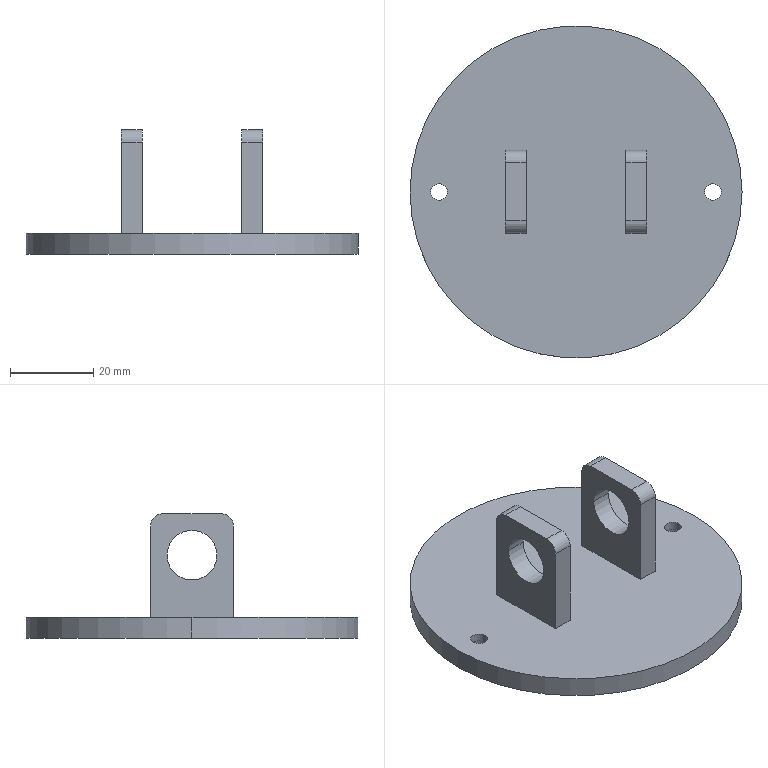Part | STEP file | Hinge seat 1 | 1 solid | 32 faces | box 80 x 80 x 30 mm | volume 28682 mm3 | cylinder 18 | plane 14 | commonest cylinder face diameters 4 x4 6 x4 7 x4 12 x4 80 x2
STEP:
#1=CARTESIAN_POINT('',(-29.5,0.,3.));
#2=VERTEX_POINT('',#1);
#3=CARTESIAN_POINT('',(-36.5,0.,3.));
#4=VERTEX_POINT('',#3);
#5=CARTESIAN_POINT('',(-33.,0.,3.));
#6=DIRECTION('',(0.,0.,-1.));
#7=DIRECTION('',(-1.,0.,0.));
#8=AXIS2_PLACEMENT_3D('',#5,#6,#7);
#9=CIRCLE('',#8,3.5);
#10=EDGE_CURVE('',#2,#4,#9,.T.);
#11=ORIENTED_EDGE('',*,*,#10,.F.);
#12=CARTESIAN_POINT('',(-29.5,0.,0.));
#13=VERTEX_POINT('',#12);
#14=CARTESIAN_POINT('',(-29.5,0.,3.));
#15=DIRECTION('',(0.,0.,-1.));
#16=VECTOR('',#15,1000.);
#17=LINE('',#14,#16);
#18=EDGE_CURVE('',#2,#13,#17,.T.);
#19=ORIENTED_EDGE('',*,*,#18,.T.);
#20=CARTESIAN_POINT('',(-36.5,0.,0.));
#21=VERTEX_POINT('',#20);
#22=CARTESIAN_POINT('',(-33.,0.,0.));
#23=DIRECTION('',(0.,0.,-1.));
#24=DIRECTION('',(-1.,0.,0.));
#25=AXIS2_PLACEMENT_3D('',#22,#23,#24);
#26=CIRCLE('',#25,3.5);
#27=EDGE_CURVE('',#13,#21,#26,.T.);
#28=ORIENTED_EDGE('',*,*,#27,.T.);
#29=CARTESIAN_POINT('',(-36.5,0.,3.));
#30=DIRECTION('',(0.,0.,-1.));
#31=VECTOR('',#30,1000.);
#32=LINE('',#29,#31);
#33=EDGE_CURVE('',#4,#21,#32,.T.);
#34=ORIENTED_EDGE('',*,*,#33,.F.);
#35=EDGE_LOOP('',(#11,#19,#28,#34));
#36=FACE_OUTER_BOUND('',#35,.T.);
#37=CARTESIAN_POINT('',(-33.,0.,3.));
#38=DIRECTION('',(0.,0.,-1.));
#39=DIRECTION('',(-1.,0.,0.));
#40=AXIS2_PLACEMENT_3D('',#37,#38,#39);
#41=CYLINDRICAL_SURFACE('',#40,3.5);
#42=ADVANCED_FACE('',(#36),#41,.F.);
#43=CARTESIAN_POINT('',(36.5,0.,3.));
#44=VERTEX_POINT('',#43);
#45=CARTESIAN_POINT('',(29.5,0.,3.));
#46=VERTEX_POINT('',#45);
#47=CARTESIAN_POINT('',(33.,0.,3.));
#48=DIRECTION('',(0.,0.,-1.));
#49=DIRECTION('',(-1.,0.,0.));
#50=AXIS2_PLACEMENT_3D('',#47,#48,#49);
#51=CIRCLE('',#50,3.5);
#52=EDGE_CURVE('',#44,#46,#51,.T.);
#53=ORIENTED_EDGE('',*,*,#52,.F.);
#54=CARTESIAN_POINT('',(36.5,0.,0.));
#55=VERTEX_POINT('',#54);
#56=CARTESIAN_POINT('',(36.5,0.,3.));
#57=DIRECTION('',(0.,0.,-1.));
#58=VECTOR('',#57,1000.);
#59=LINE('',#56,#58);
#60=EDGE_CURVE('',#44,#55,#59,.T.);
#61=ORIENTED_EDGE('',*,*,#60,.T.);
#62=CARTESIAN_POINT('',(29.5,0.,0.));
#63=VERTEX_POINT('',#62);
#64=CARTESIAN_POINT('',(33.,0.,0.));
#65=DIRECTION('',(0.,0.,-1.));
#66=DIRECTION('',(-1.,0.,0.));
#67=AXIS2_PLACEMENT_3D('',#64,#65,#66);
#68=CIRCLE('',#67,3.5);
#69=EDGE_CURVE('',#55,#63,#68,.T.);
#70=ORIENTED_EDGE('',*,*,#69,.T.);
#71=CARTESIAN_POINT('',(29.5,0.,3.));
#72=DIRECTION('',(0.,0.,-1.));
#73=VECTOR('',#72,1000.);
#74=LINE('',#71,#73);
#75=EDGE_CURVE('',#46,#63,#74,.T.);
#76=ORIENTED_EDGE('',*,*,#75,.F.);
#77=EDGE_LOOP('',(#53,#61,#70,#76));
#78=FACE_OUTER_BOUND('',#77,.T.);
#79=CARTESIAN_POINT('',(33.,0.,3.));
#80=DIRECTION('',(0.,0.,-1.));
#81=DIRECTION('',(-1.,0.,0.));
#82=AXIS2_PLACEMENT_3D('',#79,#80,#81);
#83=CYLINDRICAL_SURFACE('',#82,3.5);
#84=ADVANCED_FACE('',(#78),#83,.F.);
#85=CARTESIAN_POINT('',(-12.,6.,20.));
#86=VERTEX_POINT('',#85);
#87=CARTESIAN_POINT('',(-12.,-6.,20.));
#88=VERTEX_POINT('',#87);
#89=CARTESIAN_POINT('',(-12.,0.,20.));
#90=DIRECTION('',(-1.,0.,0.));
#91=DIRECTION('',(0.,-1.,0.));
#92=AXIS2_PLACEMENT_3D('',#89,#90,#91);
#93=CIRCLE('',#92,6.);
#94=EDGE_CURVE('',#86,#88,#93,.T.);
#95=ORIENTED_EDGE('',*,*,#94,.F.);
#96=CARTESIAN_POINT('',(-17.,6.,20.));
#97=VERTEX_POINT('',#96);
#98=CARTESIAN_POINT('',(40.,6.,20.));
#99=DIRECTION('',(-1.,0.,0.));
#100=VECTOR('',#99,1000.);
#101=LINE('',#98,#100);
#102=EDGE_CURVE('',#86,#97,#101,.T.);
#103=ORIENTED_EDGE('',*,*,#102,.T.);
#104=CARTESIAN_POINT('',(-17.,-6.,20.));
#105=VERTEX_POINT('',#104);
#106=CARTESIAN_POINT('',(-17.,0.,20.));
#107=DIRECTION('',(-1.,0.,0.));
#108=DIRECTION('',(0.,-1.,0.));
#109=AXIS2_PLACEMENT_3D('',#106,#107,#108);
#110=CIRCLE('',#109,6.);
#111=EDGE_CURVE('',#97,#105,#110,.T.);
#112=ORIENTED_EDGE('',*,*,#111,.T.);
#113=CARTESIAN_POINT('',(40.,-6.,20.));
#114=DIRECTION('',(-1.,0.,0.));
#115=VECTOR('',#114,1000.);
#116=LINE('',#113,#115);
#117=EDGE_CURVE('',#88,#105,#116,.T.);
#118=ORIENTED_EDGE('',*,*,#117,.F.);
#119=EDGE_LOOP('',(#95,#103,#112,#118));
#120=FACE_OUTER_BOUND('',#119,.T.);
#121=CARTESIAN_POINT('',(40.,0.,20.));
#122=DIRECTION('',(-1.,0.,0.));
#123=DIRECTION('',(0.,-1.,0.));
#124=AXIS2_PLACEMENT_3D('',#121,#122,#123);
#125=CYLINDRICAL_SURFACE('',#124,6.);
#126=ADVANCED_FACE('',(#120),#125,.F.);
#127=CARTESIAN_POINT('',(17.,6.,20.));
#128=VERTEX_POINT('',#127);
#129=CARTESIAN_POINT('',(17.,-6.,20.));
#130=VERTEX_POINT('',#129);
#131=CARTESIAN_POINT('',(17.,0.,20.));
#132=DIRECTION('',(-1.,0.,0.));
#133=DIRECTION('',(0.,-1.,0.));
#134=AXIS2_PLACEMENT_3D('',#131,#132,#133);
#135=CIRCLE('',#134,6.);
#136=EDGE_CURVE('',#128,#130,#135,.T.);
#137=ORIENTED_EDGE('',*,*,#136,.F.);
#138=CARTESIAN_POINT('',(12.,6.,20.));
#139=VERTEX_POINT('',#138);
#140=CARTESIAN_POINT('',(40.,6.,20.));
#141=DIRECTION('',(-1.,0.,0.));
#142=VECTOR('',#141,1000.);
#143=LINE('',#140,#142);
#144=EDGE_CURVE('',#128,#139,#143,.T.);
#145=ORIENTED_EDGE('',*,*,#144,.T.);
#146=CARTESIAN_POINT('',(12.,-6.,20.));
#147=VERTEX_POINT('',#146);
#148=CARTESIAN_POINT('',(12.,0.,20.));
#149=DIRECTION('',(1.,0.,0.));
#150=DIRECTION('',(0.,1.,0.));
#151=AXIS2_PLACEMENT_3D('',#148,#149,#150);
#152=CIRCLE('',#151,6.);
#153=EDGE_CURVE('',#147,#139,#152,.T.);
#154=ORIENTED_EDGE('',*,*,#153,.F.);
#155=CARTESIAN_POINT('',(40.,-6.,20.));
#156=DIRECTION('',(-1.,0.,0.));
#157=VECTOR('',#156,1000.);
#158=LINE('',#155,#157);
#159=EDGE_CURVE('',#130,#147,#158,.T.);
#160=ORIENTED_EDGE('',*,*,#159,.F.);
#161=EDGE_LOOP('',(#137,#145,#154,#160));
#162=FACE_OUTER_BOUND('',#161,.T.);
#163=CARTESIAN_POINT('',(40.,0.,20.));
#164=DIRECTION('',(-1.,0.,0.));
#165=DIRECTION('',(0.,-1.,0.));
#166=AXIS2_PLACEMENT_3D('',#163,#164,#165);
#167=CYLINDRICAL_SURFACE('',#166,6.);
#168=ADVANCED_FACE('',(#162),#167,.F.);
#169=CARTESIAN_POINT('',(40.,0.,5.));
#170=VERTEX_POINT('',#169);
#171=CARTESIAN_POINT('',(-40.,0.,5.));
#172=VERTEX_POINT('',#171);
#173=CARTESIAN_POINT('',(0.,0.,5.));
#174=DIRECTION('',(0.,0.,1.));
#175=DIRECTION('',(1.,0.,0.));
#176=AXIS2_PLACEMENT_3D('',#173,#174,#175);
#177=CIRCLE('',#176,40.);
#178=EDGE_CURVE('',#170,#172,#177,.T.);
#179=ORIENTED_EDGE('',*,*,#178,.F.);
#180=CARTESIAN_POINT('',(40.,0.,0.));
#181=VERTEX_POINT('',#180);
#182=CARTESIAN_POINT('',(40.,0.,5.));
#183=DIRECTION('',(0.,0.,-1.));
#184=VECTOR('',#183,1000.);
#185=LINE('',#182,#184);
#186=EDGE_CURVE('',#170,#181,#185,.T.);
#187=ORIENTED_EDGE('',*,*,#186,.T.);
#188=CARTESIAN_POINT('',(-40.,0.,0.));
#189=VERTEX_POINT('',#188);
#190=CARTESIAN_POINT('',(0.,0.,0.));
#191=DIRECTION('',(0.,0.,1.));
#192=DIRECTION('',(1.,0.,0.));
#193=AXIS2_PLACEMENT_3D('',#190,#191,#192);
#194=CIRCLE('',#193,40.);
#195=EDGE_CURVE('',#181,#189,#194,.T.);
#196=ORIENTED_EDGE('',*,*,#195,.T.);
#197=CARTESIAN_POINT('',(-40.,0.,5.));
#198=DIRECTION('',(0.,0.,-1.));
#199=VECTOR('',#198,1000.);
#200=LINE('',#197,#199);
#201=EDGE_CURVE('',#172,#189,#200,.T.);
#202=ORIENTED_EDGE('',*,*,#201,.F.);
#203=EDGE_LOOP('',(#179,#187,#196,#202));
#204=FACE_OUTER_BOUND('',#203,.T.);
#205=CARTESIAN_POINT('',(0.,0.,5.));
#206=DIRECTION('',(0.,0.,-1.));
#207=DIRECTION('',(-1.,0.,0.));
#208=AXIS2_PLACEMENT_3D('',#205,#206,#207);
#209=CYLINDRICAL_SURFACE('',#208,40.);
#210=ADVANCED_FACE('',(#204),#209,.T.);
#211=CARTESIAN_POINT('',(31.,0.,5.));
#212=VERTEX_POINT('',#211);
#213=CARTESIAN_POINT('',(35.,0.,5.));
#214=VERTEX_POINT('',#213);
#215=CARTESIAN_POINT('',(33.,0.,5.));
#216=DIRECTION('',(0.,0.,1.));
#217=DIRECTION('',(1.,0.,0.));
#218=AXIS2_PLACEMENT_3D('',#215,#216,#217);
#219=CIRCLE('',#218,2.);
#220=EDGE_CURVE('',#212,#214,#219,.T.);
#221=ORIENTED_EDGE('',*,*,#220,.T.);
#222=CARTESIAN_POINT('',(35.,0.,3.));
#223=VERTEX_POINT('',#222);
#224=CARTESIAN_POINT('',(35.,0.,30.));
#225=DIRECTION('',(0.,0.,-1.));
#226=VECTOR('',#225,1000.);
#227=LINE('',#224,#226);
#228=EDGE_CURVE('',#214,#223,#227,.T.);
#229=ORIENTED_EDGE('',*,*,#228,.T.);
#230=CARTESIAN_POINT('',(31.,0.,3.));
#231=VERTEX_POINT('',#230);
#232=CARTESIAN_POINT('',(33.,0.,3.));
#233=DIRECTION('',(0.,0.,1.));
#234=DIRECTION('',(-1.,0.,0.));
#235=AXIS2_PLACEMENT_3D('',#232,#233,#234);
#236=CIRCLE('',#235,2.);
#237=EDGE_CURVE('',#231,#223,#236,.T.);
#238=ORIENTED_EDGE('',*,*,#237,.F.);
#239=CARTESIAN_POINT('',(31.,0.,30.));
#240=DIRECTION('',(0.,0.,-1.));
#241=VECTOR('',#240,1000.);
#242=LINE('',#239,#241);
#243=EDGE_CURVE('',#212,#231,#242,.T.);
#244=ORIENTED_EDGE('',*,*,#243,.F.);
#245=EDGE_LOOP('',(#221,#229,#238,#244));
#246=FACE_OUTER_BOUND('',#245,.T.);
#247=CARTESIAN_POINT('',(33.,0.,30.));
#248=DIRECTION('',(0.,0.,-1.));
#249=DIRECTION('',(-1.,0.,0.));
#250=AXIS2_PLACEMENT_3D('',#247,#248,#249);
#251=CYLINDRICAL_SURFACE('',#250,2.);
#252=ADVANCED_FACE('',(#246),#251,.F.);
#253=CARTESIAN_POINT('',(-35.,0.,5.));
#254=VERTEX_POINT('',#253);
#255=CARTESIAN_POINT('',(-31.,0.,5.));
#256=VERTEX_POINT('',#255);
#257=CARTESIAN_POINT('',(-33.,0.,5.));
#258=DIRECTION('',(0.,0.,1.));
#259=DIRECTION('',(1.,0.,0.));
#260=AXIS2_PLACEMENT_3D('',#257,#258,#259);
#261=CIRCLE('',#260,2.);
#262=EDGE_CURVE('',#254,#256,#261,.T.);
#263=ORIENTED_EDGE('',*,*,#262,.T.);
#264=CARTESIAN_POINT('',(-31.,0.,3.));
#265=VERTEX_POINT('',#264);
#266=CARTESIAN_POINT('',(-31.,0.,30.));
#267=DIRECTION('',(0.,0.,-1.));
#268=VECTOR('',#267,1000.);
#269=LINE('',#266,#268);
#270=EDGE_CURVE('',#256,#265,#269,.T.);
#271=ORIENTED_EDGE('',*,*,#270,.T.);
#272=CARTESIAN_POINT('',(-35.,0.,3.));
#273=VERTEX_POINT('',#272);
#274=CARTESIAN_POINT('',(-33.,0.,3.));
#275=DIRECTION('',(0.,0.,1.));
#276=DIRECTION('',(-1.,0.,0.));
#277=AXIS2_PLACEMENT_3D('',#274,#275,#276);
#278=CIRCLE('',#277,2.);
#279=EDGE_CURVE('',#273,#265,#278,.T.);
#280=ORIENTED_EDGE('',*,*,#279,.F.);
#281=CARTESIAN_POINT('',(-35.,0.,30.));
#282=DIRECTION('',(0.,0.,-1.));
#283=VECTOR('',#282,1000.);
#284=LINE('',#281,#283);
#285=EDGE_CURVE('',#254,#273,#284,.T.);
#286=ORIENTED_EDGE('',*,*,#285,.F.);
#287=EDGE_LOOP('',(#263,#271,#280,#286));
#288=FACE_OUTER_BOUND('',#287,.T.);
#289=CARTESIAN_POINT('',(-33.,0.,30.));
#290=DIRECTION('',(0.,0.,-1.));
#291=DIRECTION('',(-1.,0.,0.));
#292=AXIS2_PLACEMENT_3D('',#289,#290,#291);
#293=CYLINDRICAL_SURFACE('',#292,2.);
#294=ADVANCED_FACE('',(#288),#293,.F.);
#295=ORIENTED_EDGE('',*,*,#270,.F.);
#296=CARTESIAN_POINT('',(-33.,0.,5.));
#297=DIRECTION('',(0.,0.,1.));
#298=DIRECTION('',(1.,0.,0.));
#299=AXIS2_PLACEMENT_3D('',#296,#297,#298);
#300=CIRCLE('',#299,2.);
#301=EDGE_CURVE('',#256,#254,#300,.T.);
#302=ORIENTED_EDGE('',*,*,#301,.T.);
#303=ORIENTED_EDGE('',*,*,#285,.T.);
#304=CARTESIAN_POINT('',(-33.,0.,3.));
#305=DIRECTION('',(0.,0.,1.));
#306=DIRECTION('',(-1.,0.,0.));
#307=AXIS2_PLACEMENT_3D('',#304,#305,#306);
#308=CIRCLE('',#307,2.);
#309=EDGE_CURVE('',#265,#273,#308,.T.);
#310=ORIENTED_EDGE('',*,*,#309,.F.);
#311=EDGE_LOOP('',(#295,#302,#303,#310));
#312=FACE_OUTER_BOUND('',#311,.T.);
#313=CARTESIAN_POINT('',(-33.,0.,30.));
#314=DIRECTION('',(0.,0.,-1.));
#315=DIRECTION('',(-1.,0.,0.));
#316=AXIS2_PLACEMENT_3D('',#313,#314,#315);
#317=CYLINDRICAL_SURFACE('',#316,2.);
#318=ADVANCED_FACE('',(#312),#317,.F.);
#319=ORIENTED_EDGE('',*,*,#228,.F.);
#320=CARTESIAN_POINT('',(33.,0.,5.));
#321=DIRECTION('',(0.,0.,1.));
#322=DIRECTION('',(1.,0.,0.));
#323=AXIS2_PLACEMENT_3D('',#320,#321,#322);
#324=CIRCLE('',#323,2.);
#325=EDGE_CURVE('',#214,#212,#324,.T.);
#326=ORIENTED_EDGE('',*,*,#325,.T.);
#327=ORIENTED_EDGE('',*,*,#243,.T.);
#328=CARTESIAN_POINT('',(33.,0.,3.));
#329=DIRECTION('',(0.,0.,1.));
#330=DIRECTION('',(-1.,0.,0.));
#331=AXIS2_PLACEMENT_3D('',#328,#329,#330);
#332=CIRCLE('',#331,2.);
#333=EDGE_CURVE('',#223,#231,#332,.T.);
#334=ORIENTED_EDGE('',*,*,#333,.F.);
#335=EDGE_LOOP('',(#319,#326,#327,#334));
#336=FACE_OUTER_BOUND('',#335,.T.);
#337=CARTESIAN_POINT('',(33.,0.,30.));
#338=DIRECTION('',(0.,0.,-1.));
#339=DIRECTION('',(-1.,0.,0.));
#340=AXIS2_PLACEMENT_3D('',#337,#338,#339);
#341=CYLINDRICAL_SURFACE('',#340,2.);
#342=ADVANCED_FACE('',(#336),#341,.F.);
#343=ORIENTED_EDGE('',*,*,#220,.F.);
#344=ORIENTED_EDGE('',*,*,#325,.F.);
#345=EDGE_LOOP('',(#343,#344));
#346=FACE_BOUND('',#345,.T.);
#347=ORIENTED_EDGE('',*,*,#262,.F.);
#348=ORIENTED_EDGE('',*,*,#301,.F.);
#349=EDGE_LOOP('',(#347,#348));
#350=FACE_BOUND('',#349,.T.);
#351=CARTESIAN_POINT('',(0.,0.,5.));
#352=DIRECTION('',(0.,0.,1.));
#353=DIRECTION('',(1.,0.,0.));
#354=AXIS2_PLACEMENT_3D('',#351,#352,#353);
#355=CIRCLE('',#354,40.);
#356=EDGE_CURVE('',#172,#170,#355,.T.);
#357=ORIENTED_EDGE('',*,*,#356,.T.);
#358=ORIENTED_EDGE('',*,*,#178,.T.);
#359=EDGE_LOOP('',(#357,#358));
#360=FACE_OUTER_BOUND('',#359,.T.);
#361=CARTESIAN_POINT('',(-12.,10.,5.));
#362=VERTEX_POINT('',#361);
#363=CARTESIAN_POINT('',(-17.,10.,5.));
#364=VERTEX_POINT('',#363);
#365=CARTESIAN_POINT('',(-17.,10.,5.));
#366=DIRECTION('',(-1.,0.,0.));
#367=VECTOR('',#366,1000.);
#368=LINE('',#365,#367);
#369=EDGE_CURVE('',#362,#364,#368,.T.);
#370=ORIENTED_EDGE('',*,*,#369,.F.);
#371=CARTESIAN_POINT('',(-12.,-10.,5.));
#372=VERTEX_POINT('',#371);
#373=CARTESIAN_POINT('',(-12.,10.,5.));
#374=DIRECTION('',(0.,1.,0.));
#375=VECTOR('',#374,1000.);
#376=LINE('',#373,#375);
#377=EDGE_CURVE('',#372,#362,#376,.T.);
#378=ORIENTED_EDGE('',*,*,#377,.F.);
#379=CARTESIAN_POINT('',(-17.,-10.,5.));
#380=VERTEX_POINT('',#379);
#381=CARTESIAN_POINT('',(-17.,-10.,5.));
#382=DIRECTION('',(1.,0.,0.));
#383=VECTOR('',#382,1000.);
#384=LINE('',#381,#383);
#385=EDGE_CURVE('',#380,#372,#384,.T.);
#386=ORIENTED_EDGE('',*,*,#385,.F.);
#387=CARTESIAN_POINT('',(-17.,10.,5.));
#388=DIRECTION('',(0.,-1.,0.));
#389=VECTOR('',#388,1000.);
#390=LINE('',#387,#389);
#391=EDGE_CURVE('',#364,#380,#390,.T.);
#392=ORIENTED_EDGE('',*,*,#391,.F.);
#393=EDGE_LOOP('',(#370,#378,#386,#392));
#394=FACE_BOUND('',#393,.T.);
#395=CARTESIAN_POINT('',(17.,10.,5.));
#396=VERTEX_POINT('',#395);
#397=CARTESIAN_POINT('',(12.,10.,5.));
#398=VERTEX_POINT('',#397);
#399=CARTESIAN_POINT('',(17.,10.,5.));
#400=DIRECTION('',(-1.,0.,0.));
#401=VECTOR('',#400,1000.);
#402=LINE('',#399,#401);
#403=EDGE_CURVE('',#396,#398,#402,.T.);
#404=ORIENTED_EDGE('',*,*,#403,.F.);
#405=CARTESIAN_POINT('',(17.,-10.,5.));
#406=VERTEX_POINT('',#405);
#407=CARTESIAN_POINT('',(17.,10.,5.));
#408=DIRECTION('',(0.,1.,0.));
#409=VECTOR('',#408,1000.);
#410=LINE('',#407,#409);
#411=EDGE_CURVE('',#406,#396,#410,.T.);
#412=ORIENTED_EDGE('',*,*,#411,.F.);
#413=CARTESIAN_POINT('',(12.,-10.,5.));
#414=VERTEX_POINT('',#413);
#415=CARTESIAN_POINT('',(17.,-10.,5.));
#416=DIRECTION('',(1.,0.,0.));
#417=VECTOR('',#416,1000.);
#418=LINE('',#415,#417);
#419=EDGE_CURVE('',#414,#406,#418,.T.);
#420=ORIENTED_EDGE('',*,*,#419,.F.);
#421=CARTESIAN_POINT('',(12.,10.,5.));
#422=DIRECTION('',(0.,-1.,0.));
#423=VECTOR('',#422,1000.);
#424=LINE('',#421,#423);
#425=EDGE_CURVE('',#398,#414,#424,.T.);
#426=ORIENTED_EDGE('',*,*,#425,.F.);
#427=EDGE_LOOP('',(#404,#412,#420,#426));
#428=FACE_BOUND('',#427,.T.);
#429=CARTESIAN_POINT('',(0.,0.,5.));
#430=DIRECTION('',(0.,0.,1.));
#431=DIRECTION('',(1.,0.,0.));
#432=AXIS2_PLACEMENT_3D('',#429,#430,#431);
#433=PLANE('',#432);
#434=ADVANCED_FACE('',(#346,#350,#360,#394,#428),#433,.T.);
#435=ORIENTED_EDGE('',*,*,#186,.F.);
#436=ORIENTED_EDGE('',*,*,#356,.F.);
#437=ORIENTED_EDGE('',*,*,#201,.T.);
#438=CARTESIAN_POINT('',(0.,0.,0.));
#439=DIRECTION('',(0.,0.,1.));
#440=DIRECTION('',(1.,0.,0.));
#441=AXIS2_PLACEMENT_3D('',#438,#439,#440);
#442=CIRCLE('',#441,40.);
#443=EDGE_CURVE('',#189,#181,#442,.T.);
#444=ORIENTED_EDGE('',*,*,#443,.T.);
#445=EDGE_LOOP('',(#435,#436,#437,#444));
#446=FACE_OUTER_BOUND('',#445,.T.);
#447=CARTESIAN_POINT('',(0.,0.,5.));
#448=DIRECTION('',(0.,0.,-1.));
#449=DIRECTION('',(-1.,0.,0.));
#450=AXIS2_PLACEMENT_3D('',#447,#448,#449);
#451=CYLINDRICAL_SURFACE('',#450,40.);
#452=ADVANCED_FACE('',(#446),#451,.T.);
#453=CARTESIAN_POINT('',(33.,0.,0.));
#454=DIRECTION('',(0.,0.,-1.));
#455=DIRECTION('',(-1.,0.,0.));
#456=AXIS2_PLACEMENT_3D('',#453,#454,#455);
#457=CIRCLE('',#456,3.5);
#458=EDGE_CURVE('',#63,#55,#457,.T.);
#459=ORIENTED_EDGE('',*,*,#458,.F.);
#460=ORIENTED_EDGE('',*,*,#69,.F.);
#461=EDGE_LOOP('',(#459,#460));
#462=FACE_BOUND('',#461,.T.);
#463=CARTESIAN_POINT('',(-33.,0.,0.));
#464=DIRECTION('',(0.,0.,-1.));
#465=DIRECTION('',(-1.,0.,0.));
#466=AXIS2_PLACEMENT_3D('',#463,#464,#465);
#467=CIRCLE('',#466,3.5);
#468=EDGE_CURVE('',#21,#13,#467,.T.);
#469=ORIENTED_EDGE('',*,*,#468,.F.);
#470=ORIENTED_EDGE('',*,*,#27,.F.);
#471=EDGE_LOOP('',(#469,#470));
#472=FACE_BOUND('',#471,.T.);
#473=ORIENTED_EDGE('',*,*,#443,.F.);
#474=ORIENTED_EDGE('',*,*,#195,.F.);
#475=EDGE_LOOP('',(#473,#474));
#476=FACE_OUTER_BOUND('',#475,.T.);
#477=CARTESIAN_POINT('',(0.,0.,0.));
#478=DIRECTION('',(0.,0.,1.));
#479=DIRECTION('',(1.,0.,0.));
#480=AXIS2_PLACEMENT_3D('',#477,#478,#479);
#481=PLANE('',#480);
#482=ADVANCED_FACE('',(#462,#472,#476),#481,.F.);
#483=CARTESIAN_POINT('',(-12.,0.,20.));
#484=DIRECTION('',(-1.,0.,0.));
#485=DIRECTION('',(0.,-1.,0.));
#486=AXIS2_PLACEMENT_3D('',#483,#484,#485);
#487=CIRCLE('',#486,6.);
#488=EDGE_CURVE('',#88,#86,#487,.T.);
#489=ORIENTED_EDGE('',*,*,#488,.T.);
#490=ORIENTED_EDGE('',*,*,#94,.T.);
#491=EDGE_LOOP('',(#489,#490));
#492=FACE_BOUND('',#491,.T.);
#493=CARTESIAN_POINT('',(-12.,-7.,30.));
#494=VERTEX_POINT('',#493);
#495=CARTESIAN_POINT('',(-12.,7.,30.));
#496=VERTEX_POINT('',#495);
#497=CARTESIAN_POINT('',(-12.,10.,30.));
#498=DIRECTION('',(0.,1.,0.));
#499=VECTOR('',#498,1000.);
#500=LINE('',#497,#499);
#501=EDGE_CURVE('',#494,#496,#500,.T.);
#502=ORIENTED_EDGE('',*,*,#501,.F.);
#503=CARTESIAN_POINT('',(-12.,-10.,27.));
#504=VERTEX_POINT('',#503);
#505=CARTESIAN_POINT('',(-12.,-7.,27.));
#506=DIRECTION('',(1.,0.,0.));
#507=DIRECTION('',(0.,-1.,0.));
#508=AXIS2_PLACEMENT_3D('',#505,#506,#507);
#509=CIRCLE('',#508,3.);
#510=EDGE_CURVE('',#494,#504,#509,.T.);
#511=ORIENTED_EDGE('',*,*,#510,.T.);
#512=CARTESIAN_POINT('',(-12.,-10.,30.));
#513=DIRECTION('',(0.,0.,-1.));
#514=VECTOR('',#513,1000.);
#515=LINE('',#512,#514);
#516=EDGE_CURVE('',#504,#372,#515,.T.);
#517=ORIENTED_EDGE('',*,*,#516,.T.);
#518=ORIENTED_EDGE('',*,*,#377,.T.);
#519=CARTESIAN_POINT('',(-12.,10.,27.));
#520=VERTEX_POINT('',#519);
#521=CARTESIAN_POINT('',(-12.,10.,30.));
#522=DIRECTION('',(0.,0.,-1.));
#523=VECTOR('',#522,1000.);
#524=LINE('',#521,#523);
#525=EDGE_CURVE('',#520,#362,#524,.T.);
#526=ORIENTED_EDGE('',*,*,#525,.F.);
#527=CARTESIAN_POINT('',(-12.,7.,27.));
#528=DIRECTION('',(1.,0.,0.));
#529=DIRECTION('',(0.,-1.,0.));
#530=AXIS2_PLACEMENT_3D('',#527,#528,#529);
#531=CIRCLE('',#530,3.);
#532=EDGE_CURVE('',#520,#496,#531,.T.);
#533=ORIENTED_EDGE('',*,*,#532,.T.);
#534=EDGE_LOOP('',(#502,#511,#517,#518,#526,#533));
#535=FACE_OUTER_BOUND('',#534,.T.);
#536=CARTESIAN_POINT('',(-12.,10.,30.));
#537=DIRECTION('',(-1.,0.,0.));
#538=DIRECTION('',(0.,-1.,0.));
#539=AXIS2_PLACEMENT_3D('',#536,#537,#538);
#540=PLANE('',#539);
#541=ADVANCED_FACE('',(#492,#535),#540,.F.);
#542=CARTESIAN_POINT('',(-17.,10.,27.));
#543=VERTEX_POINT('',#542);
#544=CARTESIAN_POINT('',(-17.,10.,30.));
#545=DIRECTION('',(0.,0.,-1.));
#546=VECTOR('',#545,1000.);
#547=LINE('',#544,#546);
#548=EDGE_CURVE('',#543,#364,#547,.T.);
#549=ORIENTED_EDGE('',*,*,#548,.F.);
#550=CARTESIAN_POINT('',(-12.,10.,27.));
#551=DIRECTION('',(1.,0.,0.));
#552=VECTOR('',#551,1000.);
#553=LINE('',#550,#552);
#554=EDGE_CURVE('',#543,#520,#553,.T.);
#555=ORIENTED_EDGE('',*,*,#554,.T.);
#556=ORIENTED_EDGE('',*,*,#525,.T.);
#557=ORIENTED_EDGE('',*,*,#369,.T.);
#558=EDGE_LOOP('',(#549,#555,#556,#557));
#559=FACE_OUTER_BOUND('',#558,.T.);
#560=CARTESIAN_POINT('',(-17.,10.,30.));
#561=DIRECTION('',(0.,-1.,0.));
#562=DIRECTION('',(0.,0.,-1.));
#563=AXIS2_PLACEMENT_3D('',#560,#561,#562);
#564=PLANE('',#563);
#565=ADVANCED_FACE('',(#559),#564,.F.);
#566=CARTESIAN_POINT('',(-17.,0.,20.));
#567=DIRECTION('',(-1.,0.,0.));
#568=DIRECTION('',(0.,-1.,0.));
#569=AXIS2_PLACEMENT_3D('',#566,#567,#568);
#570=CIRCLE('',#569,6.);
#571=EDGE_CURVE('',#105,#97,#570,.T.);
#572=ORIENTED_EDGE('',*,*,#571,.F.);
#573=ORIENTED_EDGE('',*,*,#111,.F.);
#574=EDGE_LOOP('',(#572,#573));
#575=FACE_BOUND('',#574,.T.);
#576=CARTESIAN_POINT('',(-17.,-10.,27.));
#577=VERTEX_POINT('',#576);
#578=CARTESIAN_POINT('',(-17.,-10.,30.));
#579=DIRECTION('',(0.,0.,-1.));
#580=VECTOR('',#579,1000.);
#581=LINE('',#578,#580);
#582=EDGE_CURVE('',#577,#380,#581,.T.);
#583=ORIENTED_EDGE('',*,*,#582,.F.);
#584=CARTESIAN_POINT('',(-17.,-7.,30.));
#585=VERTEX_POINT('',#584);
#586=CARTESIAN_POINT('',(-17.,-7.,27.));
#587=DIRECTION('',(-1.,0.,0.));
#588=DIRECTION('',(0.,0.,-1.));
#589=AXIS2_PLACEMENT_3D('',#586,#587,#588);
#590=CIRCLE('',#589,3.);
#591=EDGE_CURVE('',#577,#585,#590,.T.);
#592=ORIENTED_EDGE('',*,*,#591,.T.);
#593=CARTESIAN_POINT('',(-17.,7.,30.));
#594=VERTEX_POINT('',#593);
#595=CARTESIAN_POINT('',(-17.,10.,30.));
#596=DIRECTION('',(0.,-1.,0.));
#597=VECTOR('',#596,1000.);
#598=LINE('',#595,#597);
#599=EDGE_CURVE('',#594,#585,#598,.T.);
#600=ORIENTED_EDGE('',*,*,#599,.F.);
#601=CARTESIAN_POINT('',(-17.,7.,27.));
#602=DIRECTION('',(-1.,0.,0.));
#603=DIRECTION('',(0.,0.,-1.));
#604=AXIS2_PLACEMENT_3D('',#601,#602,#603);
#605=CIRCLE('',#604,3.);
#606=EDGE_CURVE('',#594,#543,#605,.T.);
#607=ORIENTED_EDGE('',*,*,#606,.T.);
#608=ORIENTED_EDGE('',*,*,#548,.T.);
#609=ORIENTED_EDGE('',*,*,#391,.T.);
#610=EDGE_LOOP('',(#583,#592,#600,#607,#608,#609));
#611=FACE_OUTER_BOUND('',#610,.T.);
#612=CARTESIAN_POINT('',(-17.,10.,30.));
#613=DIRECTION('',(1.,0.,0.));
#614=DIRECTION('',(0.,0.,-1.));
#615=AXIS2_PLACEMENT_3D('',#612,#613,#614);
#616=PLANE('',#615);
#617=ADVANCED_FACE('',(#575,#611),#616,.F.);
#618=ORIENTED_EDGE('',*,*,#516,.F.);
#619=CARTESIAN_POINT('',(-17.,-10.,27.));
#620=DIRECTION('',(-1.,0.,0.));
#621=VECTOR('',#620,1000.);
#622=LINE('',#619,#621);
#623=EDGE_CURVE('',#504,#577,#622,.T.);
#624=ORIENTED_EDGE('',*,*,#623,.T.);
#625=ORIENTED_EDGE('',*,*,#582,.T.);
#626=ORIENTED_EDGE('',*,*,#385,.T.);
#627=EDGE_LOOP('',(#618,#624,#625,#626));
#628=FACE_OUTER_BOUND('',#627,.T.);
#629=CARTESIAN_POINT('',(-17.,-10.,30.));
#630=DIRECTION('',(0.,1.,0.));
#631=DIRECTION('',(0.,0.,1.));
#632=AXIS2_PLACEMENT_3D('',#629,#630,#631);
#633=PLANE('',#632);
#634=ADVANCED_FACE('',(#628),#633,.F.);
#635=ORIENTED_EDGE('',*,*,#599,.T.);
#636=CARTESIAN_POINT('',(-12.,-7.,30.));
#637=DIRECTION('',(1.,0.,0.));
#638=VECTOR('',#637,1000.);
#639=LINE('',#636,#638);
#640=EDGE_CURVE('',#585,#494,#639,.T.);
#641=ORIENTED_EDGE('',*,*,#640,.T.);
#642=ORIENTED_EDGE('',*,*,#501,.T.);
#643=CARTESIAN_POINT('',(-17.,7.,30.));
#644=DIRECTION('',(-1.,0.,0.));
#645=VECTOR('',#644,1000.);
#646=LINE('',#643,#645);
#647=EDGE_CURVE('',#496,#594,#646,.T.);
#648=ORIENTED_EDGE('',*,*,#647,.T.);
#649=EDGE_LOOP('',(#635,#641,#642,#648));
#650=FACE_OUTER_BOUND('',#649,.T.);
#651=CARTESIAN_POINT('',(0.,0.,30.));
#652=DIRECTION('',(0.,0.,1.));
#653=DIRECTION('',(1.,0.,0.));
#654=AXIS2_PLACEMENT_3D('',#651,#652,#653);
#655=PLANE('',#654);
#656=ADVANCED_FACE('',(#650),#655,.T.);
#657=CARTESIAN_POINT('',(17.,0.,20.));
#658=DIRECTION('',(-1.,0.,0.));
#659=DIRECTION('',(0.,-1.,0.));
#660=AXIS2_PLACEMENT_3D('',#657,#658,#659);
#661=CIRCLE('',#660,6.);
#662=EDGE_CURVE('',#130,#128,#661,.T.);
#663=ORIENTED_EDGE('',*,*,#662,.T.);
#664=ORIENTED_EDGE('',*,*,#136,.T.);
#665=EDGE_LOOP('',(#663,#664));
#666=FACE_BOUND('',#665,.T.);
#667=CARTESIAN_POINT('',(17.,10.,27.));
#668=VERTEX_POINT('',#667);
#669=CARTESIAN_POINT('',(17.,10.,30.));
#670=DIRECTION('',(0.,0.,-1.));
#671=VECTOR('',#670,1000.);
#672=LINE('',#669,#671);
#673=EDGE_CURVE('',#668,#396,#672,.T.);
#674=ORIENTED_EDGE('',*,*,#673,.F.);
#675=CARTESIAN_POINT('',(17.,7.,30.));
#676=VERTEX_POINT('',#675);
#677=CARTESIAN_POINT('',(17.,7.,27.));
#678=DIRECTION('',(1.,0.,0.));
#679=DIRECTION('',(0.,-1.,0.));
#680=AXIS2_PLACEMENT_3D('',#677,#678,#679);
#681=CIRCLE('',#680,3.);
#682=EDGE_CURVE('',#668,#676,#681,.T.);
#683=ORIENTED_EDGE('',*,*,#682,.T.);
#684=CARTESIAN_POINT('',(17.,-7.,30.));
#685=VERTEX_POINT('',#684);
#686=CARTESIAN_POINT('',(17.,10.,30.));
#687=DIRECTION('',(0.,1.,0.));
#688=VECTOR('',#687,1000.);
#689=LINE('',#686,#688);
#690=EDGE_CURVE('',#685,#676,#689,.T.);
#691=ORIENTED_EDGE('',*,*,#690,.F.);
#692=CARTESIAN_POINT('',(17.,-10.,27.));
#693=VERTEX_POINT('',#692);
#694=CARTESIAN_POINT('',(17.,-7.,27.));
#695=DIRECTION('',(1.,0.,0.));
#696=DIRECTION('',(0.,-1.,0.));
#697=AXIS2_PLACEMENT_3D('',#694,#695,#696);
#698=CIRCLE('',#697,3.);
#699=EDGE_CURVE('',#685,#693,#698,.T.);
#700=ORIENTED_EDGE('',*,*,#699,.T.);
#701=CARTESIAN_POINT('',(17.,-10.,30.));
#702=DIRECTION('',(0.,0.,-1.));
#703=VECTOR('',#702,1000.);
#704=LINE('',#701,#703);
#705=EDGE_CURVE('',#693,#406,#704,.T.);
#706=ORIENTED_EDGE('',*,*,#705,.T.);
#707=ORIENTED_EDGE('',*,*,#411,.T.);
#708=EDGE_LOOP('',(#674,#683,#691,#700,#706,#707));
#709=FACE_OUTER_BOUND('',#708,.T.);
#710=CARTESIAN_POINT('',(17.,10.,30.));
#711=DIRECTION('',(-1.,0.,0.));
#712=DIRECTION('',(0.,-1.,0.));
#713=AXIS2_PLACEMENT_3D('',#710,#711,#712);
#714=PLANE('',#713);
#715=ADVANCED_FACE('',(#666,#709),#714,.F.);
#716=CARTESIAN_POINT('',(12.,10.,27.));
#717=VERTEX_POINT('',#716);
#718=CARTESIAN_POINT('',(12.,10.,30.));
#719=DIRECTION('',(0.,0.,-1.));
#720=VECTOR('',#719,1000.);
#721=LINE('',#718,#720);
#722=EDGE_CURVE('',#717,#398,#721,.T.);
#723=ORIENTED_EDGE('',*,*,#722,.F.);
#724=CARTESIAN_POINT('',(17.,10.,27.));
#725=DIRECTION('',(1.,0.,0.));
#726=VECTOR('',#725,1000.);
#727=LINE('',#724,#726);
#728=EDGE_CURVE('',#717,#668,#727,.T.);
#729=ORIENTED_EDGE('',*,*,#728,.T.);
#730=ORIENTED_EDGE('',*,*,#673,.T.);
#731=ORIENTED_EDGE('',*,*,#403,.T.);
#732=EDGE_LOOP('',(#723,#729,#730,#731));
#733=FACE_OUTER_BOUND('',#732,.T.);
#734=CARTESIAN_POINT('',(17.,10.,30.));
#735=DIRECTION('',(0.,-1.,0.));
#736=DIRECTION('',(0.,0.,-1.));
#737=AXIS2_PLACEMENT_3D('',#734,#735,#736);
#738=PLANE('',#737);
#739=ADVANCED_FACE('',(#733),#738,.F.);
#740=ORIENTED_EDGE('',*,*,#153,.T.);
#741=CARTESIAN_POINT('',(12.,0.,20.));
#742=DIRECTION('',(1.,0.,0.));
#743=DIRECTION('',(0.,1.,0.));
#744=AXIS2_PLACEMENT_3D('',#741,#742,#743);
#745=CIRCLE('',#744,6.);
#746=EDGE_CURVE('',#139,#147,#745,.T.);
#747=ORIENTED_EDGE('',*,*,#746,.T.);
#748=EDGE_LOOP('',(#740,#747));
#749=FACE_BOUND('',#748,.T.);
#750=CARTESIAN_POINT('',(12.,7.,30.));
#751=VERTEX_POINT('',#750);
#752=CARTESIAN_POINT('',(12.,-7.,30.));
#753=VERTEX_POINT('',#752);
#754=CARTESIAN_POINT('',(12.,10.,30.));
#755=DIRECTION('',(0.,-1.,0.));
#756=VECTOR('',#755,1000.);
#757=LINE('',#754,#756);
#758=EDGE_CURVE('',#751,#753,#757,.T.);
#759=ORIENTED_EDGE('',*,*,#758,.F.);
#760=CARTESIAN_POINT('',(12.,7.,27.));
#761=DIRECTION('',(-1.,0.,0.));
#762=DIRECTION('',(0.,1.,0.));
#763=AXIS2_PLACEMENT_3D('',#760,#761,#762);
#764=CIRCLE('',#763,3.);
#765=EDGE_CURVE('',#751,#717,#764,.T.);
#766=ORIENTED_EDGE('',*,*,#765,.T.);
#767=ORIENTED_EDGE('',*,*,#722,.T.);
#768=ORIENTED_EDGE('',*,*,#425,.T.);
#769=CARTESIAN_POINT('',(12.,-10.,27.));
#770=VERTEX_POINT('',#769);
#771=CARTESIAN_POINT('',(12.,-10.,30.));
#772=DIRECTION('',(0.,0.,-1.));
#773=VECTOR('',#772,1000.);
#774=LINE('',#771,#773);
#775=EDGE_CURVE('',#770,#414,#774,.T.);
#776=ORIENTED_EDGE('',*,*,#775,.F.);
#777=CARTESIAN_POINT('',(12.,-7.,27.));
#778=DIRECTION('',(-1.,0.,0.));
#779=DIRECTION('',(0.,1.,0.));
#780=AXIS2_PLACEMENT_3D('',#777,#778,#779);
#781=CIRCLE('',#780,3.);
#782=EDGE_CURVE('',#770,#753,#781,.T.);
#783=ORIENTED_EDGE('',*,*,#782,.T.);
#784=EDGE_LOOP('',(#759,#766,#767,#768,#776,#783));
#785=FACE_OUTER_BOUND('',#784,.T.);
#786=CARTESIAN_POINT('',(12.,10.,30.));
#787=DIRECTION('',(1.,0.,0.));
#788=DIRECTION('',(0.,1.,0.));
#789=AXIS2_PLACEMENT_3D('',#786,#787,#788);
#790=PLANE('',#789);
#791=ADVANCED_FACE('',(#749,#785),#790,.F.);
#792=ORIENTED_EDGE('',*,*,#705,.F.);
#793=CARTESIAN_POINT('',(17.,-10.,27.));
#794=DIRECTION('',(-1.,0.,0.));
#795=VECTOR('',#794,1000.);
#796=LINE('',#793,#795);
#797=EDGE_CURVE('',#693,#770,#796,.T.);
#798=ORIENTED_EDGE('',*,*,#797,.T.);
#799=ORIENTED_EDGE('',*,*,#775,.T.);
#800=ORIENTED_EDGE('',*,*,#419,.T.);
#801=EDGE_LOOP('',(#792,#798,#799,#800));
#802=FACE_OUTER_BOUND('',#801,.T.);
#803=CARTESIAN_POINT('',(17.,-10.,30.));
#804=DIRECTION('',(0.,1.,0.));
#805=DIRECTION('',(0.,0.,1.));
#806=AXIS2_PLACEMENT_3D('',#803,#804,#805);
#807=PLANE('',#806);
#808=ADVANCED_FACE('',(#802),#807,.F.);
#809=ORIENTED_EDGE('',*,*,#690,.T.);
#810=CARTESIAN_POINT('',(0.,7.,30.));
#811=DIRECTION('',(-1.,0.,0.));
#812=VECTOR('',#811,1000.);
#813=LINE('',#810,#812);
#814=EDGE_CURVE('',#676,#751,#813,.T.);
#815=ORIENTED_EDGE('',*,*,#814,.T.);
#816=ORIENTED_EDGE('',*,*,#758,.T.);
#817=CARTESIAN_POINT('',(0.,-7.,30.));
#818=DIRECTION('',(1.,0.,0.));
#819=VECTOR('',#818,1000.);
#820=LINE('',#817,#819);
#821=EDGE_CURVE('',#753,#685,#820,.T.);
#822=ORIENTED_EDGE('',*,*,#821,.T.);
#823=EDGE_LOOP('',(#809,#815,#816,#822));
#824=FACE_OUTER_BOUND('',#823,.T.);
#825=CARTESIAN_POINT('',(0.,0.,30.));
#826=DIRECTION('',(0.,0.,-1.));
#827=DIRECTION('',(-1.,0.,0.));
#828=AXIS2_PLACEMENT_3D('',#825,#826,#827);
#829=PLANE('',#828);
#830=ADVANCED_FACE('',(#824),#829,.F.);
#831=ORIENTED_EDGE('',*,*,#682,.F.);
#832=ORIENTED_EDGE('',*,*,#728,.F.);
#833=ORIENTED_EDGE('',*,*,#765,.F.);
#834=ORIENTED_EDGE('',*,*,#814,.F.);
#835=EDGE_LOOP('',(#831,#832,#833,#834));
#836=FACE_OUTER_BOUND('',#835,.T.);
#837=CARTESIAN_POINT('',(0.,7.,27.));
#838=DIRECTION('',(-1.,0.,0.));
#839=DIRECTION('',(0.,0.,1.));
#840=AXIS2_PLACEMENT_3D('',#837,#838,#839);
#841=CYLINDRICAL_SURFACE('',#840,3.);
#842=ADVANCED_FACE('',(#836),#841,.T.);
#843=ORIENTED_EDGE('',*,*,#782,.F.);
#844=ORIENTED_EDGE('',*,*,#797,.F.);
#845=ORIENTED_EDGE('',*,*,#699,.F.);
#846=ORIENTED_EDGE('',*,*,#821,.F.);
#847=EDGE_LOOP('',(#843,#844,#845,#846));
#848=FACE_OUTER_BOUND('',#847,.T.);
#849=CARTESIAN_POINT('',(0.,-7.,27.));
#850=DIRECTION('',(1.,0.,0.));
#851=DIRECTION('',(0.,0.,-1.));
#852=AXIS2_PLACEMENT_3D('',#849,#850,#851);
#853=CYLINDRICAL_SURFACE('',#852,3.);
#854=ADVANCED_FACE('',(#848),#853,.T.);
#855=ORIENTED_EDGE('',*,*,#591,.F.);
#856=ORIENTED_EDGE('',*,*,#623,.F.);
#857=ORIENTED_EDGE('',*,*,#510,.F.);
#858=ORIENTED_EDGE('',*,*,#640,.F.);
#859=EDGE_LOOP('',(#855,#856,#857,#858));
#860=FACE_OUTER_BOUND('',#859,.T.);
#861=CARTESIAN_POINT('',(0.,-7.,27.));
#862=DIRECTION('',(-1.,0.,0.));
#863=DIRECTION('',(0.,0.,1.));
#864=AXIS2_PLACEMENT_3D('',#861,#862,#863);
#865=CYLINDRICAL_SURFACE('',#864,3.);
#866=ADVANCED_FACE('',(#860),#865,.T.);
#867=ORIENTED_EDGE('',*,*,#532,.F.);
#868=ORIENTED_EDGE('',*,*,#554,.F.);
#869=ORIENTED_EDGE('',*,*,#606,.F.);
#870=ORIENTED_EDGE('',*,*,#647,.F.);
#871=EDGE_LOOP('',(#867,#868,#869,#870));
#872=FACE_OUTER_BOUND('',#871,.T.);
#873=CARTESIAN_POINT('',(0.,7.,27.));
#874=DIRECTION('',(1.,0.,0.));
#875=DIRECTION('',(0.,0.,-1.));
#876=AXIS2_PLACEMENT_3D('',#873,#874,#875);
#877=CYLINDRICAL_SURFACE('',#876,3.);
#878=ADVANCED_FACE('',(#872),#877,.T.);
#879=ORIENTED_EDGE('',*,*,#144,.F.);
#880=ORIENTED_EDGE('',*,*,#662,.F.);
#881=ORIENTED_EDGE('',*,*,#159,.T.);
#882=ORIENTED_EDGE('',*,*,#746,.F.);
#883=EDGE_LOOP('',(#879,#880,#881,#882));
#884=FACE_OUTER_BOUND('',#883,.T.);
#885=CARTESIAN_POINT('',(40.,0.,20.));
#886=DIRECTION('',(-1.,0.,0.));
#887=DIRECTION('',(0.,-1.,0.));
#888=AXIS2_PLACEMENT_3D('',#885,#886,#887);
#889=CYLINDRICAL_SURFACE('',#888,6.);
#890=ADVANCED_FACE('',(#884),#889,.F.);
#891=ORIENTED_EDGE('',*,*,#102,.F.);
#892=ORIENTED_EDGE('',*,*,#488,.F.);
#893=ORIENTED_EDGE('',*,*,#117,.T.);
#894=ORIENTED_EDGE('',*,*,#571,.T.);
#895=EDGE_LOOP('',(#891,#892,#893,#894));
#896=FACE_OUTER_BOUND('',#895,.T.);
#897=CARTESIAN_POINT('',(40.,0.,20.));
#898=DIRECTION('',(-1.,0.,0.));
#899=DIRECTION('',(0.,-1.,0.));
#900=AXIS2_PLACEMENT_3D('',#897,#898,#899);
#901=CYLINDRICAL_SURFACE('',#900,6.);
#902=ADVANCED_FACE('',(#896),#901,.F.);
#903=CARTESIAN_POINT('',(33.,0.,3.));
#904=DIRECTION('',(0.,0.,-1.));
#905=DIRECTION('',(-1.,0.,0.));
#906=AXIS2_PLACEMENT_3D('',#903,#904,#905);
#907=CIRCLE('',#906,3.5);
#908=EDGE_CURVE('',#46,#44,#907,.T.);
#909=ORIENTED_EDGE('',*,*,#908,.T.);
#910=ORIENTED_EDGE('',*,*,#52,.T.);
#911=EDGE_LOOP('',(#909,#910));
#912=FACE_OUTER_BOUND('',#911,.T.);
#913=ORIENTED_EDGE('',*,*,#237,.T.);
#914=ORIENTED_EDGE('',*,*,#333,.T.);
#915=EDGE_LOOP('',(#913,#914));
#916=FACE_BOUND('',#915,.T.);
#917=CARTESIAN_POINT('',(33.,0.,3.));
#918=DIRECTION('',(0.,0.,-1.));
#919=DIRECTION('',(-1.,0.,0.));
#920=AXIS2_PLACEMENT_3D('',#917,#918,#919);
#921=PLANE('',#920);
#922=ADVANCED_FACE('',(#912,#916),#921,.T.);
#923=ORIENTED_EDGE('',*,*,#60,.F.);
#924=ORIENTED_EDGE('',*,*,#908,.F.);
#925=ORIENTED_EDGE('',*,*,#75,.T.);
#926=ORIENTED_EDGE('',*,*,#458,.T.);
#927=EDGE_LOOP('',(#923,#924,#925,#926));
#928=FACE_OUTER_BOUND('',#927,.T.);
#929=CARTESIAN_POINT('',(33.,0.,3.));
#930=DIRECTION('',(0.,0.,-1.));
#931=DIRECTION('',(-1.,0.,0.));
#932=AXIS2_PLACEMENT_3D('',#929,#930,#931);
#933=CYLINDRICAL_SURFACE('',#932,3.5);
#934=ADVANCED_FACE('',(#928),#933,.F.);
#935=CARTESIAN_POINT('',(-33.,0.,3.));
#936=DIRECTION('',(0.,0.,-1.));
#937=DIRECTION('',(-1.,0.,0.));
#938=AXIS2_PLACEMENT_3D('',#935,#936,#937);
#939=CIRCLE('',#938,3.5);
#940=EDGE_CURVE('',#4,#2,#939,.T.);
#941=ORIENTED_EDGE('',*,*,#940,.T.);
#942=ORIENTED_EDGE('',*,*,#10,.T.);
#943=EDGE_LOOP('',(#941,#942));
#944=FACE_OUTER_BOUND('',#943,.T.);
#945=ORIENTED_EDGE('',*,*,#279,.T.);
#946=ORIENTED_EDGE('',*,*,#309,.T.);
#947=EDGE_LOOP('',(#945,#946));
#948=FACE_BOUND('',#947,.T.);
#949=CARTESIAN_POINT('',(-33.,0.,3.));
#950=DIRECTION('',(0.,0.,-1.));
#951=DIRECTION('',(-1.,0.,0.));
#952=AXIS2_PLACEMENT_3D('',#949,#950,#951);
#953=PLANE('',#952);
#954=ADVANCED_FACE('',(#944,#948),#953,.T.);
#955=ORIENTED_EDGE('',*,*,#18,.F.);
#956=ORIENTED_EDGE('',*,*,#940,.F.);
#957=ORIENTED_EDGE('',*,*,#33,.T.);
#958=ORIENTED_EDGE('',*,*,#468,.T.);
#959=EDGE_LOOP('',(#955,#956,#957,#958));
#960=FACE_OUTER_BOUND('',#959,.T.);
#961=CARTESIAN_POINT('',(-33.,0.,3.));
#962=DIRECTION('',(0.,0.,-1.));
#963=DIRECTION('',(-1.,0.,0.));
#964=AXIS2_PLACEMENT_3D('',#961,#962,#963);
#965=CYLINDRICAL_SURFACE('',#964,3.5);
#966=ADVANCED_FACE('',(#960),#965,.F.);
#967=CLOSED_SHELL('',(#42,#84,#126,#168,#210,#252,#294,#318,#342,#434,#452,#482,#541,#565,#617,#634,#656,#715,#739,#791,#808,#830,#842,#854,#866,#878,#890,#902,#922,#934,#954,#966));
#968=MANIFOLD_SOLID_BREP('',#967);
#969=CARTESIAN_POINT('',(0.,0.,0.));
#970=DIRECTION('',(0.,0.,1.));
#971=DIRECTION('',(1.,0.,0.));
#972=AXIS2_PLACEMENT_3D('',#969,#970,#971);
#973=(LENGTH_UNIT()NAMED_UNIT(*)SI_UNIT(.MILLI.,.METRE.));
#974=UNCERTAINTY_MEASURE_WITH_UNIT(LENGTH_MEASURE(0.00001),#973,'','');
#975=(NAMED_UNIT(*)PLANE_ANGLE_UNIT()SI_UNIT($,.RADIAN.));
#976=(NAMED_UNIT(*)SI_UNIT($,.STERADIAN.)SOLID_ANGLE_UNIT());
#977=(GEOMETRIC_REPRESENTATION_CONTEXT(3)GLOBAL_UNCERTAINTY_ASSIGNED_CONTEXT((#974))GLOBAL_UNIT_ASSIGNED_CONTEXT((#973,#975,#976))REPRESENTATION_CONTEXT('',''));
#978=ADVANCED_BREP_SHAPE_REPRESENTATION('',(#968,#972),#977);